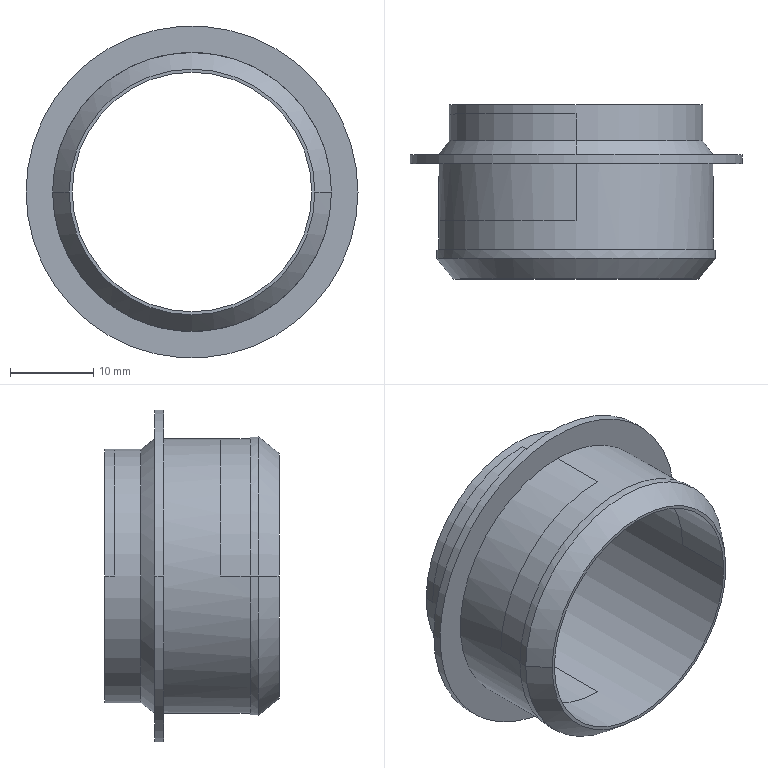Part | STEP file | 1 solid | 19 faces | box 40 x 20.98 x 40 mm | volume 3947 mm3 | cylinder 10 | plane 5 | cone 4 | commonest cylinder face diameters 28.86 x2 30.6 x2 33.1 x2 33.6 x2 40 x2
STEP:
#1=CARTESIAN_POINT('',(0.,0.,0.));
#2=DIRECTION('',(0.,0.,1.));
#3=DIRECTION('',(1.,0.,0.));
#4=AXIS2_PLACEMENT_3D('',#1,#2,#3);
#5=CARTESIAN_POINT('',(0.,16.886,16.55));
#6=VERTEX_POINT('',#5);
#7=CARTESIAN_POINT('',(16.55,16.886,0.));
#8=VERTEX_POINT('',#7);
#9=CARTESIAN_POINT('',(0.,16.886,0.));
#10=DIRECTION('',(0.,1.,0.));
#11=DIRECTION('',(0.,0.,1.));
#12=AXIS2_PLACEMENT_3D('',#9,#10,#11);
#13=CIRCLE('',#12,16.55);
#14=EDGE_CURVE('',#6,#8,#13,.T.);
#15=ORIENTED_EDGE('',*,*,#14,.F.);
#16=CARTESIAN_POINT('',(-16.55,16.886,0.));
#17=VERTEX_POINT('',#16);
#18=CARTESIAN_POINT('',(0.,16.886,0.));
#19=DIRECTION('',(0.,1.,0.));
#20=DIRECTION('',(-1.,0.,0.));
#21=AXIS2_PLACEMENT_3D('',#18,#19,#20);
#22=CIRCLE('',#21,16.55);
#23=EDGE_CURVE('',#17,#6,#22,.T.);
#24=ORIENTED_EDGE('',*,*,#23,.F.);
#25=CARTESIAN_POINT('',(-16.55,20.386,0.));
#26=VERTEX_POINT('',#25);
#27=CARTESIAN_POINT('',(-16.55,20.386,0.));
#28=DIRECTION('',(0.,-1.,0.));
#29=VECTOR('',#28,3.5);
#30=LINE('',#27,#29);
#31=EDGE_CURVE('',#26,#17,#30,.T.);
#32=ORIENTED_EDGE('',*,*,#31,.F.);
#33=CARTESIAN_POINT('',(0.,20.386,16.55));
#34=VERTEX_POINT('',#33);
#35=CARTESIAN_POINT('',(0.,20.386,0.));
#36=DIRECTION('',(0.,-1.,0.));
#37=DIRECTION('',(0.,0.,1.));
#38=AXIS2_PLACEMENT_3D('',#35,#36,#37);
#39=CIRCLE('',#38,16.55);
#40=EDGE_CURVE('',#34,#26,#39,.T.);
#41=ORIENTED_EDGE('',*,*,#40,.F.);
#42=CARTESIAN_POINT('',(0.,27.286,16.55));
#43=VERTEX_POINT('',#42);
#44=CARTESIAN_POINT('',(0.,20.386,16.55));
#45=DIRECTION('',(0.,1.,0.));
#46=VECTOR('',#45,6.9);
#47=LINE('',#44,#46);
#48=EDGE_CURVE('',#34,#43,#47,.T.);
#49=ORIENTED_EDGE('',*,*,#48,.T.);
#50=CARTESIAN_POINT('',(0.,27.286,-16.55));
#51=VERTEX_POINT('',#50);
#52=CARTESIAN_POINT('',(0.,27.286,0.));
#53=DIRECTION('',(0.,-1.,0.));
#54=DIRECTION('',(0.,0.,-1.));
#55=AXIS2_PLACEMENT_3D('',#52,#53,#54);
#56=CIRCLE('',#55,16.55);
#57=EDGE_CURVE('',#51,#43,#56,.T.);
#58=ORIENTED_EDGE('',*,*,#57,.F.);
#59=CARTESIAN_POINT('',(0.,20.386,-16.55));
#60=VERTEX_POINT('',#59);
#61=CARTESIAN_POINT('',(0.,20.386,-16.55));
#62=DIRECTION('',(0.,1.,0.));
#63=VECTOR('',#62,6.9);
#64=LINE('',#61,#63);
#65=EDGE_CURVE('',#60,#51,#64,.T.);
#66=ORIENTED_EDGE('',*,*,#65,.F.);
#67=CARTESIAN_POINT('',(16.55,20.386,0.));
#68=VERTEX_POINT('',#67);
#69=CARTESIAN_POINT('',(0.,20.386,0.));
#70=DIRECTION('',(0.,-1.,0.));
#71=DIRECTION('',(0.,0.,-1.));
#72=AXIS2_PLACEMENT_3D('',#69,#70,#71);
#73=CIRCLE('',#72,16.55);
#74=EDGE_CURVE('',#60,#68,#73,.T.);
#75=ORIENTED_EDGE('',*,*,#74,.T.);
#76=CARTESIAN_POINT('',(16.55,20.386,0.));
#77=DIRECTION('',(0.,-1.,0.));
#78=VECTOR('',#77,3.5);
#79=LINE('',#76,#78);
#80=EDGE_CURVE('',#68,#8,#79,.T.);
#81=ORIENTED_EDGE('',*,*,#80,.T.);
#82=EDGE_LOOP('',(#15,#24,#32,#41,#49,#58,#66,#75,#81));
#83=FACE_OUTER_BOUND('',#82,.F.);
#84=CARTESIAN_POINT('',(0.,0.,0.));
#85=DIRECTION('',(0.,-1.,0.));
#86=DIRECTION('',(0.,0.,-1.));
#87=AXIS2_PLACEMENT_3D('',#84,#85,#86);
#88=CYLINDRICAL_SURFACE('',#87,16.55);
#89=ADVANCED_FACE('',(#83),#88,.T.);
#90=CARTESIAN_POINT('',(16.8,16.886,0.));
#91=VERTEX_POINT('',#90);
#92=CARTESIAN_POINT('',(-16.8,16.886,0.));
#93=VERTEX_POINT('',#92);
#94=CARTESIAN_POINT('',(0.,16.886,0.));
#95=DIRECTION('',(0.,-1.,0.));
#96=DIRECTION('',(1.,0.,0.));
#97=AXIS2_PLACEMENT_3D('',#94,#95,#96);
#98=CIRCLE('',#97,16.8);
#99=EDGE_CURVE('',#91,#93,#98,.T.);
#100=ORIENTED_EDGE('',*,*,#99,.T.);
#101=CARTESIAN_POINT('',(0.,16.886,0.));
#102=DIRECTION('',(0.,-1.,0.));
#103=DIRECTION('',(-1.,0.,0.));
#104=AXIS2_PLACEMENT_3D('',#101,#102,#103);
#105=CIRCLE('',#104,16.8);
#106=EDGE_CURVE('',#93,#91,#105,.T.);
#107=ORIENTED_EDGE('',*,*,#106,.T.);
#108=EDGE_LOOP('',(#100,#107));
#109=FACE_OUTER_BOUND('',#108,.F.);
#110=ORIENTED_EDGE('',*,*,#23,.T.);
#111=ORIENTED_EDGE('',*,*,#14,.T.);
#112=CARTESIAN_POINT('',(0.,16.886,-16.55));
#113=VERTEX_POINT('',#112);
#114=CARTESIAN_POINT('',(0.,16.886,0.));
#115=DIRECTION('',(0.,1.,0.));
#116=DIRECTION('',(1.,0.,0.));
#117=AXIS2_PLACEMENT_3D('',#114,#115,#116);
#118=CIRCLE('',#117,16.55);
#119=EDGE_CURVE('',#8,#113,#118,.T.);
#120=ORIENTED_EDGE('',*,*,#119,.T.);
#121=CARTESIAN_POINT('',(0.,16.886,0.));
#122=DIRECTION('',(0.,1.,0.));
#123=DIRECTION('',(0.,0.,-1.));
#124=AXIS2_PLACEMENT_3D('',#121,#122,#123);
#125=CIRCLE('',#124,16.55);
#126=EDGE_CURVE('',#113,#17,#125,.T.);
#127=ORIENTED_EDGE('',*,*,#126,.T.);
#128=EDGE_LOOP('',(#110,#111,#120,#127));
#129=FACE_BOUND('',#128,.F.);
#130=CARTESIAN_POINT('',(0.,16.886,0.));
#131=DIRECTION('',(0.,-1.,0.));
#132=DIRECTION('',(1.,0.,0.));
#133=AXIS2_PLACEMENT_3D('',#130,#131,#132);
#134=PLANE('',#133);
#135=ADVANCED_FACE('',(#109,#129),#134,.F.);
#136=CARTESIAN_POINT('',(0.,15.886,16.8));
#137=VERTEX_POINT('',#136);
#138=CARTESIAN_POINT('',(16.8,15.886,0.));
#139=VERTEX_POINT('',#138);
#140=CARTESIAN_POINT('',(0.,15.886,0.));
#141=DIRECTION('',(0.,1.,0.));
#142=DIRECTION('',(0.,0.,1.));
#143=AXIS2_PLACEMENT_3D('',#140,#141,#142);
#144=CIRCLE('',#143,16.8);
#145=EDGE_CURVE('',#137,#139,#144,.T.);
#146=ORIENTED_EDGE('',*,*,#145,.F.);
#147=CARTESIAN_POINT('',(-16.8,15.886,-0.000000001));
#148=VERTEX_POINT('',#147);
#149=CARTESIAN_POINT('',(0.,15.886,0.));
#150=DIRECTION('',(0.,1.,0.));
#151=DIRECTION('',(-1.,0.,0.));
#152=AXIS2_PLACEMENT_3D('',#149,#150,#151);
#153=CIRCLE('',#152,16.8);
#154=EDGE_CURVE('',#148,#137,#153,.T.);
#155=ORIENTED_EDGE('',*,*,#154,.F.);
#156=CARTESIAN_POINT('',(-16.8,16.886,0.));
#157=DIRECTION('',(0.,-1.,0.));
#158=VECTOR('',#157,1.);
#159=LINE('',#156,#158);
#160=EDGE_CURVE('',#93,#148,#159,.T.);
#161=ORIENTED_EDGE('',*,*,#160,.F.);
#162=ORIENTED_EDGE('',*,*,#99,.F.);
#163=CARTESIAN_POINT('',(16.8,16.886,0.));
#164=DIRECTION('',(0.,-1.,0.));
#165=VECTOR('',#164,1.);
#166=LINE('',#163,#165);
#167=EDGE_CURVE('',#91,#139,#166,.T.);
#168=ORIENTED_EDGE('',*,*,#167,.T.);
#169=EDGE_LOOP('',(#146,#155,#161,#162,#168));
#170=FACE_OUTER_BOUND('',#169,.F.);
#171=CARTESIAN_POINT('',(0.,16.886,0.));
#172=DIRECTION('',(0.,-1.,0.));
#173=DIRECTION('',(1.,0.,0.));
#174=AXIS2_PLACEMENT_3D('',#171,#172,#173);
#175=CYLINDRICAL_SURFACE('',#174,16.8);
#176=ADVANCED_FACE('',(#170),#175,.T.);
#177=CARTESIAN_POINT('',(0.,13.386,14.8));
#178=VERTEX_POINT('',#177);
#179=CARTESIAN_POINT('',(14.8,13.386,0.));
#180=VERTEX_POINT('',#179);
#181=CARTESIAN_POINT('',(0.,13.386,0.));
#182=DIRECTION('',(0.,1.,0.));
#183=DIRECTION('',(0.,0.,1.));
#184=AXIS2_PLACEMENT_3D('',#181,#182,#183);
#185=CIRCLE('',#184,14.8);
#186=EDGE_CURVE('',#178,#180,#185,.T.);
#187=ORIENTED_EDGE('',*,*,#186,.F.);
#188=CARTESIAN_POINT('',(-14.8,13.386,0.));
#189=VERTEX_POINT('',#188);
#190=CARTESIAN_POINT('',(0.,13.386,0.));
#191=DIRECTION('',(0.,1.,0.));
#192=DIRECTION('',(-1.,0.,0.));
#193=AXIS2_PLACEMENT_3D('',#190,#191,#192);
#194=CIRCLE('',#193,14.8);
#195=EDGE_CURVE('',#189,#178,#194,.T.);
#196=ORIENTED_EDGE('',*,*,#195,.F.);
#197=CARTESIAN_POINT('',(-14.8,13.386,-0.000000001));
#198=DIRECTION('',(-0.6247,0.7809,0.));
#199=VECTOR('',#198,3.202);
#200=LINE('',#197,#199);
#201=EDGE_CURVE('',#189,#148,#200,.T.);
#202=ORIENTED_EDGE('',*,*,#201,.T.);
#203=ORIENTED_EDGE('',*,*,#154,.T.);
#204=ORIENTED_EDGE('',*,*,#145,.T.);
#205=CARTESIAN_POINT('',(14.8,13.386,0.));
#206=DIRECTION('',(0.6247,0.7809,0.));
#207=VECTOR('',#206,3.202);
#208=LINE('',#205,#207);
#209=EDGE_CURVE('',#180,#139,#208,.T.);
#210=ORIENTED_EDGE('',*,*,#209,.F.);
#211=EDGE_LOOP('',(#187,#196,#202,#203,#204,#210));
#212=FACE_OUTER_BOUND('',#211,.F.);
#213=CARTESIAN_POINT('',(0.,14.636,0.));
#214=DIRECTION('',(0.,1.,0.));
#215=DIRECTION('',(0.,0.,-1.));
#216=AXIS2_PLACEMENT_3D('',#213,#214,#215);
#217=CONICAL_SURFACE('',#216,15.8,38.66);
#218=ADVANCED_FACE('',(#212),#217,.T.);
#219=ORIENTED_EDGE('',*,*,#195,.T.);
#220=ORIENTED_EDGE('',*,*,#186,.T.);
#221=CARTESIAN_POINT('',(0.,13.386,-14.8));
#222=VERTEX_POINT('',#221);
#223=CARTESIAN_POINT('',(0.,13.386,0.));
#224=DIRECTION('',(0.,1.,0.));
#225=DIRECTION('',(1.,0.,0.));
#226=AXIS2_PLACEMENT_3D('',#223,#224,#225);
#227=CIRCLE('',#226,14.8);
#228=EDGE_CURVE('',#180,#222,#227,.T.);
#229=ORIENTED_EDGE('',*,*,#228,.T.);
#230=CARTESIAN_POINT('',(0.,13.386,0.));
#231=DIRECTION('',(0.,1.,0.));
#232=DIRECTION('',(0.,0.,-1.));
#233=AXIS2_PLACEMENT_3D('',#230,#231,#232);
#234=CIRCLE('',#233,14.8);
#235=EDGE_CURVE('',#222,#189,#234,.T.);
#236=ORIENTED_EDGE('',*,*,#235,.T.);
#237=EDGE_LOOP('',(#219,#220,#229,#236));
#238=FACE_OUTER_BOUND('',#237,.F.);
#239=CARTESIAN_POINT('',(-14.43,13.386,0.));
#240=VERTEX_POINT('',#239);
#241=CARTESIAN_POINT('',(0.,13.386,-14.43));
#242=VERTEX_POINT('',#241);
#243=CARTESIAN_POINT('',(0.,13.386,0.));
#244=DIRECTION('',(0.,-1.,0.));
#245=DIRECTION('',(-1.,0.,0.));
#246=AXIS2_PLACEMENT_3D('',#243,#244,#245);
#247=CIRCLE('',#246,14.43);
#248=EDGE_CURVE('',#240,#242,#247,.T.);
#249=ORIENTED_EDGE('',*,*,#248,.T.);
#250=CARTESIAN_POINT('',(14.43,13.386,0.));
#251=VERTEX_POINT('',#250);
#252=CARTESIAN_POINT('',(0.,13.386,0.));
#253=DIRECTION('',(0.,-1.,0.));
#254=DIRECTION('',(0.,0.,-1.));
#255=AXIS2_PLACEMENT_3D('',#252,#253,#254);
#256=CIRCLE('',#255,14.43);
#257=EDGE_CURVE('',#242,#251,#256,.T.);
#258=ORIENTED_EDGE('',*,*,#257,.T.);
#259=CARTESIAN_POINT('',(0.,13.386,14.43));
#260=VERTEX_POINT('',#259);
#261=CARTESIAN_POINT('',(0.,13.386,0.));
#262=DIRECTION('',(0.,-1.,0.));
#263=DIRECTION('',(1.,0.,0.));
#264=AXIS2_PLACEMENT_3D('',#261,#262,#263);
#265=CIRCLE('',#264,14.43);
#266=EDGE_CURVE('',#251,#260,#265,.T.);
#267=ORIENTED_EDGE('',*,*,#266,.T.);
#268=CARTESIAN_POINT('',(0.,13.386,0.));
#269=DIRECTION('',(0.,-1.,0.));
#270=DIRECTION('',(0.,0.,1.));
#271=AXIS2_PLACEMENT_3D('',#268,#269,#270);
#272=CIRCLE('',#271,14.43);
#273=EDGE_CURVE('',#260,#240,#272,.T.);
#274=ORIENTED_EDGE('',*,*,#273,.T.);
#275=EDGE_LOOP('',(#249,#258,#267,#274));
#276=FACE_BOUND('',#275,.F.);
#277=CARTESIAN_POINT('',(0.,13.386,0.));
#278=DIRECTION('',(0.,-1.,0.));
#279=DIRECTION('',(1.,0.,0.));
#280=AXIS2_PLACEMENT_3D('',#277,#278,#279);
#281=PLANE('',#280);
#282=ADVANCED_FACE('',(#238,#276),#281,.T.);
#283=ORIENTED_EDGE('',*,*,#235,.F.);
#284=ORIENTED_EDGE('',*,*,#228,.F.);
#285=ORIENTED_EDGE('',*,*,#209,.T.);
#286=CARTESIAN_POINT('',(0.,15.886,-16.8));
#287=VERTEX_POINT('',#286);
#288=CARTESIAN_POINT('',(0.,15.886,0.));
#289=DIRECTION('',(0.,1.,0.));
#290=DIRECTION('',(1.,0.,0.));
#291=AXIS2_PLACEMENT_3D('',#288,#289,#290);
#292=CIRCLE('',#291,16.8);
#293=EDGE_CURVE('',#139,#287,#292,.T.);
#294=ORIENTED_EDGE('',*,*,#293,.T.);
#295=CARTESIAN_POINT('',(0.,15.886,0.));
#296=DIRECTION('',(0.,1.,0.));
#297=DIRECTION('',(0.,0.,-1.));
#298=AXIS2_PLACEMENT_3D('',#295,#296,#297);
#299=CIRCLE('',#298,16.8);
#300=EDGE_CURVE('',#287,#148,#299,.T.);
#301=ORIENTED_EDGE('',*,*,#300,.T.);
#302=ORIENTED_EDGE('',*,*,#201,.F.);
#303=EDGE_LOOP('',(#283,#284,#285,#294,#301,#302));
#304=FACE_OUTER_BOUND('',#303,.F.);
#305=CARTESIAN_POINT('',(0.,14.636,0.));
#306=DIRECTION('',(0.,1.,0.));
#307=DIRECTION('',(0.,0.,-1.));
#308=AXIS2_PLACEMENT_3D('',#305,#306,#307);
#309=CONICAL_SURFACE('',#308,15.8,38.66);
#310=ADVANCED_FACE('',(#304),#309,.T.);
#311=ORIENTED_EDGE('',*,*,#300,.F.);
#312=ORIENTED_EDGE('',*,*,#293,.F.);
#313=ORIENTED_EDGE('',*,*,#167,.F.);
#314=ORIENTED_EDGE('',*,*,#106,.F.);
#315=ORIENTED_EDGE('',*,*,#160,.T.);
#316=EDGE_LOOP('',(#311,#312,#313,#314,#315));
#317=FACE_OUTER_BOUND('',#316,.F.);
#318=CARTESIAN_POINT('',(0.,16.886,0.));
#319=DIRECTION('',(0.,-1.,0.));
#320=DIRECTION('',(1.,0.,0.));
#321=AXIS2_PLACEMENT_3D('',#318,#319,#320);
#322=CYLINDRICAL_SURFACE('',#321,16.8);
#323=ADVANCED_FACE('',(#317),#322,.T.);
#324=CARTESIAN_POINT('',(0.,20.386,-14.43));
#325=VERTEX_POINT('',#324);
#326=CARTESIAN_POINT('',(0.,33.266,-14.43));
#327=VERTEX_POINT('',#326);
#328=CARTESIAN_POINT('',(0.,20.386,-14.43));
#329=DIRECTION('',(0.,1.,0.));
#330=VECTOR('',#329,12.88);
#331=LINE('',#328,#330);
#332=EDGE_CURVE('',#325,#327,#331,.T.);
#333=ORIENTED_EDGE('',*,*,#332,.T.);
#334=CARTESIAN_POINT('',(-14.43,33.266,0.));
#335=VERTEX_POINT('',#334);
#336=CARTESIAN_POINT('',(0.,33.266,0.));
#337=DIRECTION('',(0.,1.,0.));
#338=DIRECTION('',(0.,0.,-1.));
#339=AXIS2_PLACEMENT_3D('',#336,#337,#338);
#340=CIRCLE('',#339,14.43);
#341=EDGE_CURVE('',#327,#335,#340,.T.);
#342=ORIENTED_EDGE('',*,*,#341,.T.);
#343=CARTESIAN_POINT('',(-14.43,34.366,0.));
#344=VERTEX_POINT('',#343);
#345=CARTESIAN_POINT('',(-14.43,33.266,0.));
#346=DIRECTION('',(0.,1.,0.));
#347=VECTOR('',#346,1.1);
#348=LINE('',#345,#347);
#349=EDGE_CURVE('',#335,#344,#348,.T.);
#350=ORIENTED_EDGE('',*,*,#349,.T.);
#351=CARTESIAN_POINT('',(0.,34.366,-14.43));
#352=VERTEX_POINT('',#351);
#353=CARTESIAN_POINT('',(0.,34.366,0.));
#354=DIRECTION('',(0.,1.,0.));
#355=DIRECTION('',(0.,0.,-1.));
#356=AXIS2_PLACEMENT_3D('',#353,#354,#355);
#357=CIRCLE('',#356,14.43);
#358=EDGE_CURVE('',#352,#344,#357,.T.);
#359=ORIENTED_EDGE('',*,*,#358,.F.);
#360=CARTESIAN_POINT('',(14.43,34.366,0.));
#361=VERTEX_POINT('',#360);
#362=CARTESIAN_POINT('',(0.,34.366,0.));
#363=DIRECTION('',(0.,1.,0.));
#364=DIRECTION('',(1.,0.,0.));
#365=AXIS2_PLACEMENT_3D('',#362,#363,#364);
#366=CIRCLE('',#365,14.43);
#367=EDGE_CURVE('',#361,#352,#366,.T.);
#368=ORIENTED_EDGE('',*,*,#367,.F.);
#369=CARTESIAN_POINT('',(14.43,33.266,0.));
#370=VERTEX_POINT('',#369);
#371=CARTESIAN_POINT('',(14.43,33.266,0.));
#372=DIRECTION('',(0.,1.,0.));
#373=VECTOR('',#372,1.1);
#374=LINE('',#371,#373);
#375=EDGE_CURVE('',#370,#361,#374,.T.);
#376=ORIENTED_EDGE('',*,*,#375,.F.);
#377=CARTESIAN_POINT('',(0.,33.266,14.43));
#378=VERTEX_POINT('',#377);
#379=CARTESIAN_POINT('',(0.,33.266,0.));
#380=DIRECTION('',(0.,1.,0.));
#381=DIRECTION('',(0.,0.,1.));
#382=AXIS2_PLACEMENT_3D('',#379,#380,#381);
#383=CIRCLE('',#382,14.43);
#384=EDGE_CURVE('',#378,#370,#383,.T.);
#385=ORIENTED_EDGE('',*,*,#384,.F.);
#386=CARTESIAN_POINT('',(0.,20.386,14.43));
#387=VERTEX_POINT('',#386);
#388=CARTESIAN_POINT('',(0.,20.386,14.43));
#389=DIRECTION('',(0.,1.,0.));
#390=VECTOR('',#389,12.88);
#391=LINE('',#388,#390);
#392=EDGE_CURVE('',#387,#378,#391,.T.);
#393=ORIENTED_EDGE('',*,*,#392,.F.);
#394=CARTESIAN_POINT('',(14.43,20.386,0.));
#395=VERTEX_POINT('',#394);
#396=CARTESIAN_POINT('',(0.,20.386,0.));
#397=DIRECTION('',(0.,-1.,0.));
#398=DIRECTION('',(1.,0.,0.));
#399=AXIS2_PLACEMENT_3D('',#396,#397,#398);
#400=CIRCLE('',#399,14.43);
#401=EDGE_CURVE('',#395,#387,#400,.T.);
#402=ORIENTED_EDGE('',*,*,#401,.F.);
#403=CARTESIAN_POINT('',(14.43,13.386,0.));
#404=DIRECTION('',(0.,1.,0.));
#405=VECTOR('',#404,7.);
#406=LINE('',#403,#405);
#407=EDGE_CURVE('',#251,#395,#406,.T.);
#408=ORIENTED_EDGE('',*,*,#407,.F.);
#409=ORIENTED_EDGE('',*,*,#257,.F.);
#410=ORIENTED_EDGE('',*,*,#248,.F.);
#411=CARTESIAN_POINT('',(-14.43,20.386,0.));
#412=VERTEX_POINT('',#411);
#413=CARTESIAN_POINT('',(-14.43,20.386,0.));
#414=DIRECTION('',(0.,-1.,0.));
#415=VECTOR('',#414,7.);
#416=LINE('',#413,#415);
#417=EDGE_CURVE('',#412,#240,#416,.T.);
#418=ORIENTED_EDGE('',*,*,#417,.F.);
#419=CARTESIAN_POINT('',(0.,20.386,0.));
#420=DIRECTION('',(0.,-1.,0.));
#421=DIRECTION('',(-1.,0.,0.));
#422=AXIS2_PLACEMENT_3D('',#419,#420,#421);
#423=CIRCLE('',#422,14.43);
#424=EDGE_CURVE('',#412,#325,#423,.T.);
#425=ORIENTED_EDGE('',*,*,#424,.T.);
#426=EDGE_LOOP('',(#333,#342,#350,#359,#368,#376,#385,#393,#402,#408,#409,#410,#418,#425));
#427=FACE_OUTER_BOUND('',#426,.F.);
#428=CARTESIAN_POINT('',(0.,0.,0.));
#429=DIRECTION('',(0.,-1.,0.));
#430=DIRECTION('',(0.,0.,-1.));
#431=AXIS2_PLACEMENT_3D('',#428,#429,#430);
#432=CYLINDRICAL_SURFACE('',#431,14.43);
#433=ADVANCED_FACE('',(#427),#432,.F.);
#434=ORIENTED_EDGE('',*,*,#392,.T.);
#435=ORIENTED_EDGE('',*,*,#384,.T.);
#436=ORIENTED_EDGE('',*,*,#375,.T.);
#437=CARTESIAN_POINT('',(0.,34.366,14.43));
#438=VERTEX_POINT('',#437);
#439=CARTESIAN_POINT('',(0.,34.366,0.));
#440=DIRECTION('',(0.,1.,0.));
#441=DIRECTION('',(0.,0.,1.));
#442=AXIS2_PLACEMENT_3D('',#439,#440,#441);
#443=CIRCLE('',#442,14.43);
#444=EDGE_CURVE('',#438,#361,#443,.T.);
#445=ORIENTED_EDGE('',*,*,#444,.F.);
#446=CARTESIAN_POINT('',(0.,34.366,0.));
#447=DIRECTION('',(0.,1.,0.));
#448=DIRECTION('',(-1.,0.,0.));
#449=AXIS2_PLACEMENT_3D('',#446,#447,#448);
#450=CIRCLE('',#449,14.43);
#451=EDGE_CURVE('',#344,#438,#450,.T.);
#452=ORIENTED_EDGE('',*,*,#451,.F.);
#453=ORIENTED_EDGE('',*,*,#349,.F.);
#454=ORIENTED_EDGE('',*,*,#341,.F.);
#455=ORIENTED_EDGE('',*,*,#332,.F.);
#456=ORIENTED_EDGE('',*,*,#424,.F.);
#457=ORIENTED_EDGE('',*,*,#417,.T.);
#458=ORIENTED_EDGE('',*,*,#273,.F.);
#459=ORIENTED_EDGE('',*,*,#266,.F.);
#460=ORIENTED_EDGE('',*,*,#407,.T.);
#461=ORIENTED_EDGE('',*,*,#401,.T.);
#462=EDGE_LOOP('',(#434,#435,#436,#445,#452,#453,#454,#455,#456,#457,#458,#459,#460,#461));
#463=FACE_OUTER_BOUND('',#462,.F.);
#464=CARTESIAN_POINT('',(0.,0.,0.));
#465=DIRECTION('',(0.,-1.,0.));
#466=DIRECTION('',(0.,0.,-1.));
#467=AXIS2_PLACEMENT_3D('',#464,#465,#466);
#468=CYLINDRICAL_SURFACE('',#467,14.43);
#469=ADVANCED_FACE('',(#463),#468,.F.);
#470=CARTESIAN_POINT('',(15.3,34.366,0.));
#471=VERTEX_POINT('',#470);
#472=CARTESIAN_POINT('',(0.,34.366,15.3));
#473=VERTEX_POINT('',#472);
#474=CARTESIAN_POINT('',(0.,34.366,0.));
#475=DIRECTION('',(0.,-1.,0.));
#476=DIRECTION('',(1.,0.,0.));
#477=AXIS2_PLACEMENT_3D('',#474,#475,#476);
#478=CIRCLE('',#477,15.3);
#479=EDGE_CURVE('',#471,#473,#478,.T.);
#480=ORIENTED_EDGE('',*,*,#479,.T.);
#481=CARTESIAN_POINT('',(-15.3,34.366,0.));
#482=VERTEX_POINT('',#481);
#483=CARTESIAN_POINT('',(0.,34.366,0.));
#484=DIRECTION('',(0.,-1.,0.));
#485=DIRECTION('',(0.,0.,1.));
#486=AXIS2_PLACEMENT_3D('',#483,#484,#485);
#487=CIRCLE('',#486,15.3);
#488=EDGE_CURVE('',#473,#482,#487,.T.);
#489=ORIENTED_EDGE('',*,*,#488,.T.);
#490=CARTESIAN_POINT('',(0.,34.366,-15.3));
#491=VERTEX_POINT('',#490);
#492=CARTESIAN_POINT('',(0.,34.366,0.));
#493=DIRECTION('',(0.,-1.,0.));
#494=DIRECTION('',(-1.,0.,0.));
#495=AXIS2_PLACEMENT_3D('',#492,#493,#494);
#496=CIRCLE('',#495,15.3);
#497=EDGE_CURVE('',#482,#491,#496,.T.);
#498=ORIENTED_EDGE('',*,*,#497,.T.);
#499=CARTESIAN_POINT('',(0.,34.366,0.));
#500=DIRECTION('',(0.,-1.,0.));
#501=DIRECTION('',(0.,0.,-1.));
#502=AXIS2_PLACEMENT_3D('',#499,#500,#501);
#503=CIRCLE('',#502,15.3);
#504=EDGE_CURVE('',#491,#471,#503,.T.);
#505=ORIENTED_EDGE('',*,*,#504,.T.);
#506=EDGE_LOOP('',(#480,#489,#498,#505));
#507=FACE_OUTER_BOUND('',#506,.F.);
#508=ORIENTED_EDGE('',*,*,#367,.T.);
#509=ORIENTED_EDGE('',*,*,#358,.T.);
#510=ORIENTED_EDGE('',*,*,#451,.T.);
#511=ORIENTED_EDGE('',*,*,#444,.T.);
#512=EDGE_LOOP('',(#508,#509,#510,#511));
#513=FACE_BOUND('',#512,.F.);
#514=CARTESIAN_POINT('',(0.,34.366,0.));
#515=DIRECTION('',(0.,1.,0.));
#516=DIRECTION('',(-1.,0.,0.));
#517=AXIS2_PLACEMENT_3D('',#514,#515,#516);
#518=PLANE('',#517);
#519=ADVANCED_FACE('',(#507,#513),#518,.T.);
#520=CARTESIAN_POINT('',(0.,30.026,15.3));
#521=VERTEX_POINT('',#520);
#522=CARTESIAN_POINT('',(0.,33.266,15.3));
#523=VERTEX_POINT('',#522);
#524=CARTESIAN_POINT('',(0.,30.026,15.3));
#525=DIRECTION('',(0.,1.,0.));
#526=VECTOR('',#525,3.24);
#527=LINE('',#524,#526);
#528=EDGE_CURVE('',#521,#523,#527,.T.);
#529=ORIENTED_EDGE('',*,*,#528,.T.);
#530=CARTESIAN_POINT('',(-15.3,33.266,0.));
#531=VERTEX_POINT('',#530);
#532=CARTESIAN_POINT('',(0.,33.266,0.));
#533=DIRECTION('',(0.,1.,0.));
#534=DIRECTION('',(-1.,0.,0.));
#535=AXIS2_PLACEMENT_3D('',#532,#533,#534);
#536=CIRCLE('',#535,15.3);
#537=EDGE_CURVE('',#531,#523,#536,.T.);
#538=ORIENTED_EDGE('',*,*,#537,.F.);
#539=CARTESIAN_POINT('',(-15.3,33.266,0.));
#540=DIRECTION('',(0.,1.,0.));
#541=VECTOR('',#540,1.1);
#542=LINE('',#539,#541);
#543=EDGE_CURVE('',#531,#482,#542,.T.);
#544=ORIENTED_EDGE('',*,*,#543,.T.);
#545=ORIENTED_EDGE('',*,*,#488,.F.);
#546=ORIENTED_EDGE('',*,*,#479,.F.);
#547=CARTESIAN_POINT('',(15.3,33.266,0.));
#548=VERTEX_POINT('',#547);
#549=CARTESIAN_POINT('',(15.3,33.266,0.));
#550=DIRECTION('',(0.,1.,0.));
#551=VECTOR('',#550,1.1);
#552=LINE('',#549,#551);
#553=EDGE_CURVE('',#548,#471,#552,.T.);
#554=ORIENTED_EDGE('',*,*,#553,.F.);
#555=CARTESIAN_POINT('',(0.,33.266,-15.3));
#556=VERTEX_POINT('',#555);
#557=CARTESIAN_POINT('',(0.,33.266,0.));
#558=DIRECTION('',(0.,1.,0.));
#559=DIRECTION('',(1.,0.,0.));
#560=AXIS2_PLACEMENT_3D('',#557,#558,#559);
#561=CIRCLE('',#560,15.3);
#562=EDGE_CURVE('',#548,#556,#561,.T.);
#563=ORIENTED_EDGE('',*,*,#562,.T.);
#564=CARTESIAN_POINT('',(0.,30.026,-15.3));
#565=VERTEX_POINT('',#564);
#566=CARTESIAN_POINT('',(0.,30.026,-15.3));
#567=DIRECTION('',(0.,1.,0.));
#568=VECTOR('',#567,3.24);
#569=LINE('',#566,#568);
#570=EDGE_CURVE('',#565,#556,#569,.T.);
#571=ORIENTED_EDGE('',*,*,#570,.F.);
#572=CARTESIAN_POINT('',(0.,30.026,0.));
#573=DIRECTION('',(0.,1.,0.));
#574=DIRECTION('',(0.,0.,1.));
#575=AXIS2_PLACEMENT_3D('',#572,#573,#574);
#576=CIRCLE('',#575,15.3);
#577=EDGE_CURVE('',#521,#565,#576,.T.);
#578=ORIENTED_EDGE('',*,*,#577,.F.);
#579=EDGE_LOOP('',(#529,#538,#544,#545,#546,#554,#563,#571,#578));
#580=FACE_OUTER_BOUND('',#579,.F.);
#581=CARTESIAN_POINT('',(0.,0.,0.));
#582=DIRECTION('',(0.,-1.,0.));
#583=DIRECTION('',(0.,0.,-1.));
#584=AXIS2_PLACEMENT_3D('',#581,#582,#583);
#585=CYLINDRICAL_SURFACE('',#584,15.3);
#586=ADVANCED_FACE('',(#580),#585,.T.);
#587=ORIENTED_EDGE('',*,*,#570,.T.);
#588=ORIENTED_EDGE('',*,*,#562,.F.);
#589=ORIENTED_EDGE('',*,*,#553,.T.);
#590=ORIENTED_EDGE('',*,*,#504,.F.);
#591=ORIENTED_EDGE('',*,*,#497,.F.);
#592=ORIENTED_EDGE('',*,*,#543,.F.);
#593=ORIENTED_EDGE('',*,*,#537,.T.);
#594=ORIENTED_EDGE('',*,*,#528,.F.);
#595=CARTESIAN_POINT('',(0.,30.026,0.));
#596=DIRECTION('',(0.,1.,0.));
#597=DIRECTION('',(0.,0.,-1.));
#598=AXIS2_PLACEMENT_3D('',#595,#596,#597);
#599=CIRCLE('',#598,15.3);
#600=EDGE_CURVE('',#565,#521,#599,.T.);
#601=ORIENTED_EDGE('',*,*,#600,.F.);
#602=EDGE_LOOP('',(#587,#588,#589,#590,#591,#592,#593,#594,#601));
#603=FACE_OUTER_BOUND('',#602,.F.);
#604=CARTESIAN_POINT('',(0.,0.,0.));
#605=DIRECTION('',(0.,-1.,0.));
#606=DIRECTION('',(0.,0.,-1.));
#607=AXIS2_PLACEMENT_3D('',#604,#605,#606);
#608=CYLINDRICAL_SURFACE('',#607,15.3);
#609=ADVANCED_FACE('',(#603),#608,.T.);
#610=CARTESIAN_POINT('',(0.,28.366,16.55));
#611=VERTEX_POINT('',#610);
#612=CARTESIAN_POINT('',(0.,28.366,16.55));
#613=DIRECTION('',(0.,0.7988,-0.6015));
#614=VECTOR('',#613,2.078);
#615=LINE('',#612,#614);
#616=EDGE_CURVE('',#611,#521,#615,.T.);
#617=ORIENTED_EDGE('',*,*,#616,.F.);
#618=CARTESIAN_POINT('',(0.,28.366,-16.55));
#619=VERTEX_POINT('',#618);
#620=CARTESIAN_POINT('',(0.,28.366,0.));
#621=DIRECTION('',(0.,1.,0.));
#622=DIRECTION('',(0.,0.,-1.));
#623=AXIS2_PLACEMENT_3D('',#620,#621,#622);
#624=CIRCLE('',#623,16.55);
#625=EDGE_CURVE('',#619,#611,#624,.T.);
#626=ORIENTED_EDGE('',*,*,#625,.F.);
#627=CARTESIAN_POINT('',(0.,28.366,-16.55));
#628=DIRECTION('',(0.,0.7988,0.6015));
#629=VECTOR('',#628,2.078);
#630=LINE('',#627,#629);
#631=EDGE_CURVE('',#619,#565,#630,.T.);
#632=ORIENTED_EDGE('',*,*,#631,.T.);
#633=ORIENTED_EDGE('',*,*,#600,.T.);
#634=EDGE_LOOP('',(#617,#626,#632,#633));
#635=FACE_OUTER_BOUND('',#634,.F.);
#636=CARTESIAN_POINT('',(0.,29.196,0.));
#637=DIRECTION('',(0.,-1.,0.));
#638=DIRECTION('',(0.,0.,-1.));
#639=AXIS2_PLACEMENT_3D('',#636,#637,#638);
#640=CONICAL_SURFACE('',#639,15.925,36.98);
#641=ADVANCED_FACE('',(#635),#640,.T.);
#642=ORIENTED_EDGE('',*,*,#577,.T.);
#643=ORIENTED_EDGE('',*,*,#631,.F.);
#644=CARTESIAN_POINT('',(0.,28.366,0.));
#645=DIRECTION('',(0.,1.,0.));
#646=DIRECTION('',(0.,0.,1.));
#647=AXIS2_PLACEMENT_3D('',#644,#645,#646);
#648=CIRCLE('',#647,16.55);
#649=EDGE_CURVE('',#611,#619,#648,.T.);
#650=ORIENTED_EDGE('',*,*,#649,.F.);
#651=ORIENTED_EDGE('',*,*,#616,.T.);
#652=EDGE_LOOP('',(#642,#643,#650,#651));
#653=FACE_OUTER_BOUND('',#652,.F.);
#654=CARTESIAN_POINT('',(0.,29.196,0.));
#655=DIRECTION('',(0.,-1.,0.));
#656=DIRECTION('',(0.,0.,-1.));
#657=AXIS2_PLACEMENT_3D('',#654,#655,#656);
#658=CONICAL_SURFACE('',#657,15.925,36.98);
#659=ADVANCED_FACE('',(#653),#658,.T.);
#660=CARTESIAN_POINT('',(20.,28.366,0.));
#661=VERTEX_POINT('',#660);
#662=CARTESIAN_POINT('',(-20.,28.366,0.));
#663=VERTEX_POINT('',#662);
#664=CARTESIAN_POINT('',(0.,28.366,0.));
#665=DIRECTION('',(0.,-1.,0.));
#666=DIRECTION('',(1.,0.,0.));
#667=AXIS2_PLACEMENT_3D('',#664,#665,#666);
#668=CIRCLE('',#667,20.);
#669=EDGE_CURVE('',#661,#663,#668,.T.);
#670=ORIENTED_EDGE('',*,*,#669,.T.);
#671=CARTESIAN_POINT('',(0.,28.366,0.));
#672=DIRECTION('',(0.,-1.,0.));
#673=DIRECTION('',(-1.,0.,0.));
#674=AXIS2_PLACEMENT_3D('',#671,#672,#673);
#675=CIRCLE('',#674,20.);
#676=EDGE_CURVE('',#663,#661,#675,.T.);
#677=ORIENTED_EDGE('',*,*,#676,.T.);
#678=EDGE_LOOP('',(#670,#677));
#679=FACE_OUTER_BOUND('',#678,.F.);
#680=ORIENTED_EDGE('',*,*,#649,.T.);
#681=ORIENTED_EDGE('',*,*,#625,.T.);
#682=EDGE_LOOP('',(#680,#681));
#683=FACE_BOUND('',#682,.F.);
#684=CARTESIAN_POINT('',(16.55,28.366,0.));
#685=DIRECTION('',(0.,1.,0.));
#686=DIRECTION('',(0.,0.,1.));
#687=AXIS2_PLACEMENT_3D('',#684,#685,#686);
#688=PLANE('',#687);
#689=ADVANCED_FACE('',(#679,#683),#688,.T.);
#690=ORIENTED_EDGE('',*,*,#669,.F.);
#691=CARTESIAN_POINT('',(20.,27.286,0.));
#692=VERTEX_POINT('',#691);
#693=CARTESIAN_POINT('',(20.,28.366,0.));
#694=DIRECTION('',(0.,-1.,0.));
#695=VECTOR('',#694,1.08);
#696=LINE('',#693,#695);
#697=EDGE_CURVE('',#661,#692,#696,.T.);
#698=ORIENTED_EDGE('',*,*,#697,.T.);
#699=CARTESIAN_POINT('',(-20.,27.286,0.));
#700=VERTEX_POINT('',#699);
#701=CARTESIAN_POINT('',(0.,27.286,0.));
#702=DIRECTION('',(0.,1.,0.));
#703=DIRECTION('',(-1.,0.,0.));
#704=AXIS2_PLACEMENT_3D('',#701,#702,#703);
#705=CIRCLE('',#704,20.);
#706=EDGE_CURVE('',#700,#692,#705,.T.);
#707=ORIENTED_EDGE('',*,*,#706,.F.);
#708=CARTESIAN_POINT('',(-20.,28.366,0.));
#709=DIRECTION('',(0.,-1.,0.));
#710=VECTOR('',#709,1.08);
#711=LINE('',#708,#710);
#712=EDGE_CURVE('',#663,#700,#711,.T.);
#713=ORIENTED_EDGE('',*,*,#712,.F.);
#714=EDGE_LOOP('',(#690,#698,#707,#713));
#715=FACE_OUTER_BOUND('',#714,.F.);
#716=CARTESIAN_POINT('',(0.,28.366,0.));
#717=DIRECTION('',(0.,1.,0.));
#718=DIRECTION('',(-1.,0.,0.));
#719=AXIS2_PLACEMENT_3D('',#716,#717,#718);
#720=CYLINDRICAL_SURFACE('',#719,20.);
#721=ADVANCED_FACE('',(#715),#720,.T.);
#722=ORIENTED_EDGE('',*,*,#676,.F.);
#723=ORIENTED_EDGE('',*,*,#712,.T.);
#724=CARTESIAN_POINT('',(0.,27.286,0.));
#725=DIRECTION('',(0.,1.,0.));
#726=DIRECTION('',(1.,0.,0.));
#727=AXIS2_PLACEMENT_3D('',#724,#725,#726);
#728=CIRCLE('',#727,20.);
#729=EDGE_CURVE('',#692,#700,#728,.T.);
#730=ORIENTED_EDGE('',*,*,#729,.F.);
#731=ORIENTED_EDGE('',*,*,#697,.F.);
#732=EDGE_LOOP('',(#722,#723,#730,#731));
#733=FACE_OUTER_BOUND('',#732,.F.);
#734=CARTESIAN_POINT('',(0.,28.366,0.));
#735=DIRECTION('',(0.,1.,0.));
#736=DIRECTION('',(-1.,0.,0.));
#737=AXIS2_PLACEMENT_3D('',#734,#735,#736);
#738=CYLINDRICAL_SURFACE('',#737,20.);
#739=ADVANCED_FACE('',(#733),#738,.T.);
#740=ORIENTED_EDGE('',*,*,#706,.T.);
#741=ORIENTED_EDGE('',*,*,#729,.T.);
#742=EDGE_LOOP('',(#740,#741));
#743=FACE_OUTER_BOUND('',#742,.F.);
#744=ORIENTED_EDGE('',*,*,#57,.T.);
#745=CARTESIAN_POINT('',(0.,27.286,0.));
#746=DIRECTION('',(0.,-1.,0.));
#747=DIRECTION('',(0.,0.,1.));
#748=AXIS2_PLACEMENT_3D('',#745,#746,#747);
#749=CIRCLE('',#748,16.55);
#750=EDGE_CURVE('',#43,#51,#749,.T.);
#751=ORIENTED_EDGE('',*,*,#750,.T.);
#752=EDGE_LOOP('',(#744,#751));
#753=FACE_BOUND('',#752,.F.);
#754=CARTESIAN_POINT('',(18.55,27.286,0.));
#755=DIRECTION('',(0.,-1.,0.));
#756=DIRECTION('',(0.,0.,-1.));
#757=AXIS2_PLACEMENT_3D('',#754,#755,#756);
#758=PLANE('',#757);
#759=ADVANCED_FACE('',(#743,#753),#758,.T.);
#760=ORIENTED_EDGE('',*,*,#126,.F.);
#761=ORIENTED_EDGE('',*,*,#119,.F.);
#762=ORIENTED_EDGE('',*,*,#80,.F.);
#763=ORIENTED_EDGE('',*,*,#74,.F.);
#764=ORIENTED_EDGE('',*,*,#65,.T.);
#765=ORIENTED_EDGE('',*,*,#750,.F.);
#766=ORIENTED_EDGE('',*,*,#48,.F.);
#767=ORIENTED_EDGE('',*,*,#40,.T.);
#768=ORIENTED_EDGE('',*,*,#31,.T.);
#769=EDGE_LOOP('',(#760,#761,#762,#763,#764,#765,#766,#767,#768));
#770=FACE_OUTER_BOUND('',#769,.F.);
#771=CARTESIAN_POINT('',(0.,0.,0.));
#772=DIRECTION('',(0.,-1.,0.));
#773=DIRECTION('',(0.,0.,-1.));
#774=AXIS2_PLACEMENT_3D('',#771,#772,#773);
#775=CYLINDRICAL_SURFACE('',#774,16.55);
#776=ADVANCED_FACE('',(#770),#775,.T.);
#777=CLOSED_SHELL('',(#89,#135,#176,#218,#282,#310,#323,#433,#469,#519,#586,#609,#641,#659,#689,#721,#739,#759,#776));
#778=MANIFOLD_SOLID_BREP('',#777);
#779=(LENGTH_UNIT()NAMED_UNIT(*)SI_UNIT(.MILLI.,.METRE.));
#780=UNCERTAINTY_MEASURE_WITH_UNIT(LENGTH_MEASURE(0.006035),#779,'','');
#781=(NAMED_UNIT(*)PLANE_ANGLE_UNIT()SI_UNIT($,.RADIAN.));
#782=PLANE_ANGLE_MEASURE_WITH_UNIT(PLANE_ANGLE_MEASURE(0.01745),#781);
#783=(CONVERSION_BASED_UNIT('DEGREE',#782)NAMED_UNIT(*)PLANE_ANGLE_UNIT());
#784=(NAMED_UNIT(*)SI_UNIT($,.STERADIAN.)SOLID_ANGLE_UNIT());
#785=(GEOMETRIC_REPRESENTATION_CONTEXT(3)GLOBAL_UNCERTAINTY_ASSIGNED_CONTEXT((#780))GLOBAL_UNIT_ASSIGNED_CONTEXT((#779,#783,#784))REPRESENTATION_CONTEXT('',''));
#786=ADVANCED_BREP_SHAPE_REPRESENTATION('',(#4,#778),#785);